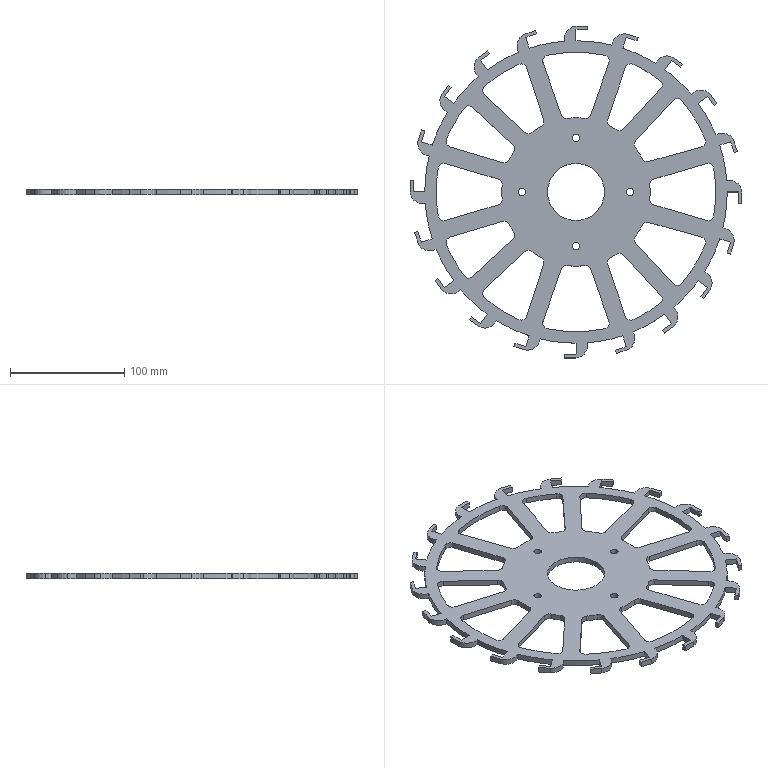Part | SolidWorks | features ICE 2, Extrusion 1, Fillet 1 | 1 solid | 247 faces | box 291 x 291 x 5 mm | volume 163158 mm3 | cylinder 141 | plane 106 | commonest cylinder face diameters 10 x60 22 x25 265 x20 130 x13 245 x13 6.5 x8